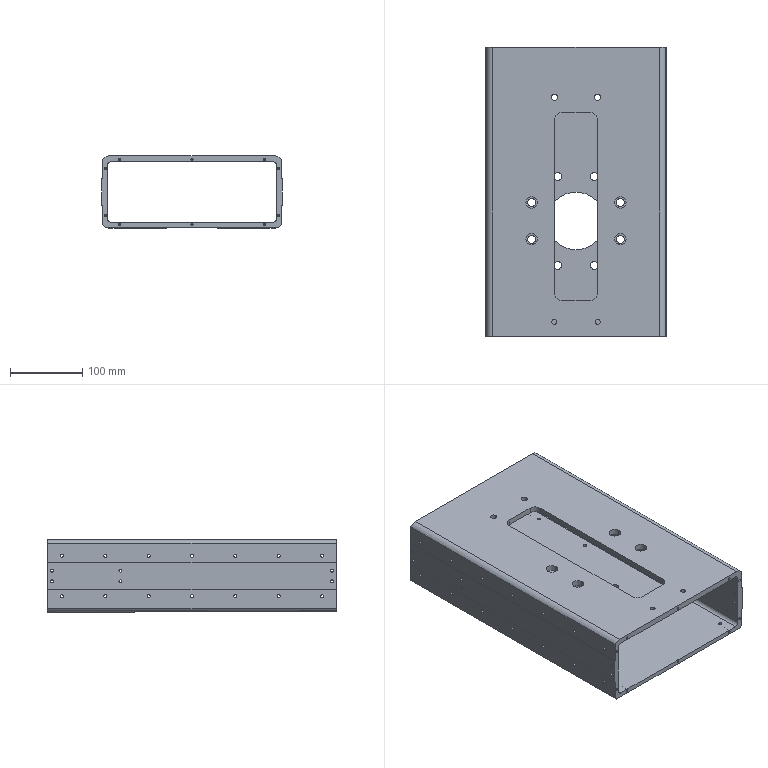Part | SolidWorks | features HoleWzd 10, Fillet 3, ICE 3, Cut 2, Extrusion 1, MirrorPattern 1 | 1 solid | 265 faces | box 250 x 400 x 100 mm | volume 1758243 mm3 | cylinder 194 | cone 40 | plane 31 | commonest cylinder face diameters 4.2 x92 3.3 x40 11 x16 5 x12 16 x8 20 x8